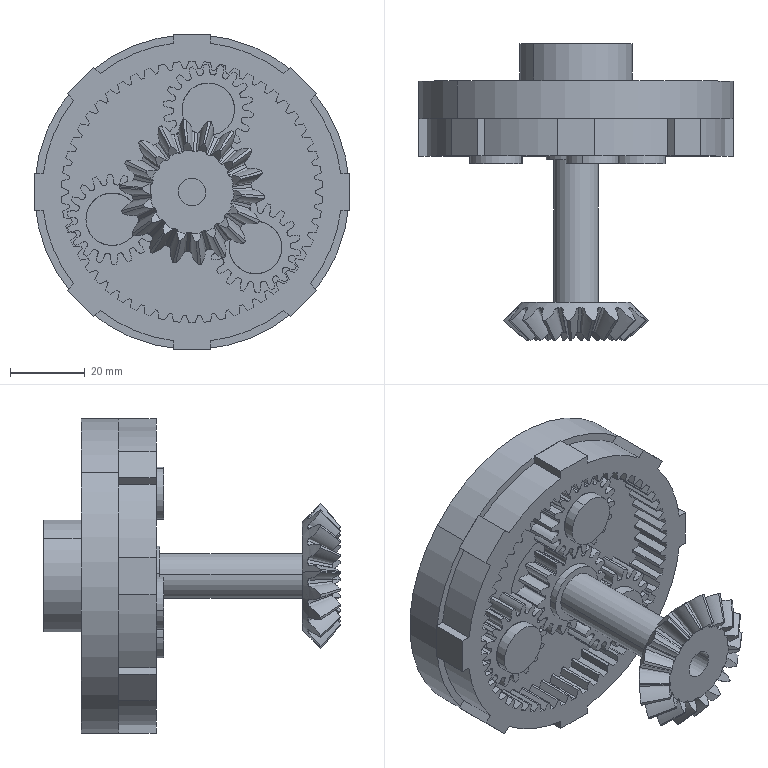Part | SolidWorks | features CompositeCurve 17 | 13 solids | 795 faces | box 84 x 79.158 x 84 mm | volume 93250 mm3 | cylinder 349 | spline 320 | plane 86 | cone 40 | commonest cylinder face diameters 24.125 x57 69.75 x55 18.5 x54 65.875 x54 12 x24 25.875 x19